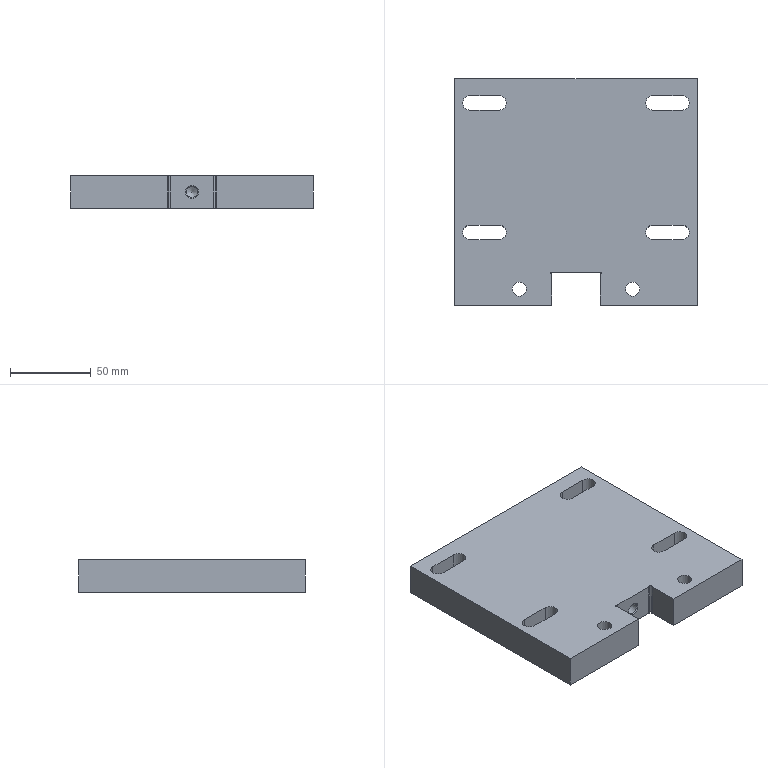Part | STEP file | YBQDJ-PD-1 | 1 solid | 41 faces | box 150 x 140 x 20 mm | volume 385255 mm3 | plane 20 | cylinder 19 | cone 2 | commonest cylinder face diameters 9 x8 4 x4 1 x2 8.7 x2 14 x2 6.8 x1